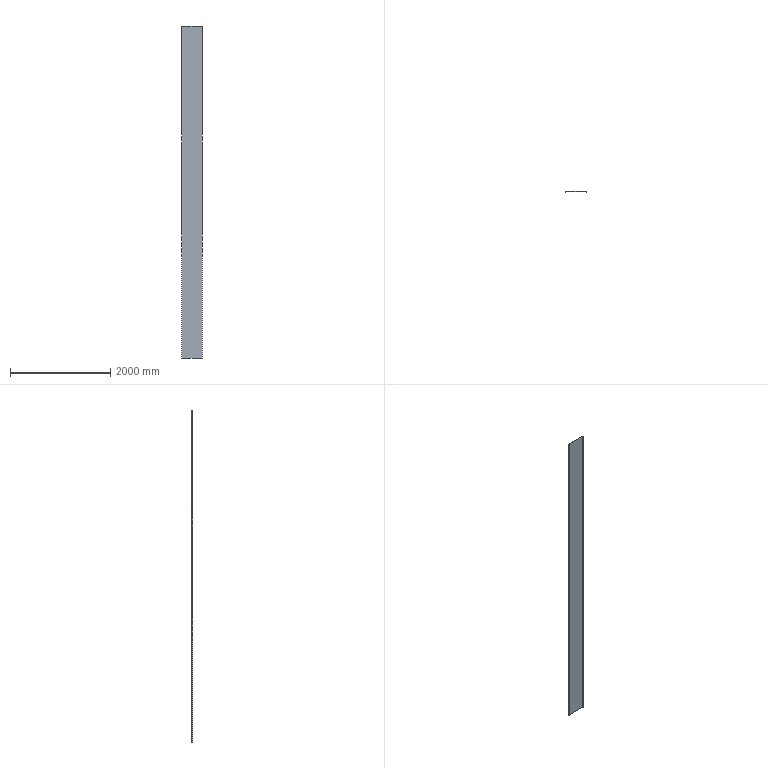Part | STEP file | 750038235 | 1 solid | 14 faces | box 405 x 21.5 x 6614 mm | volume 4395351 mm3 | plane 10 | cylinder 4 | commonest cylinder face diameters 3 x2 6 x2
STEP:
#1=CARTESIAN_POINT('',(-199.5,0.,0.));
#2=VERTEX_POINT('',#1);
#3=CARTESIAN_POINT('',(-199.5,0.,6613.5));
#4=VERTEX_POINT('',#3);
#5=CARTESIAN_POINT('',(-199.5,0.,0.));
#6=DIRECTION('',(0.,0.,1.));
#7=VECTOR('',#6,1000.);
#8=LINE('',#5,#7);
#9=EDGE_CURVE('',#2,#4,#8,.T.);
#10=ORIENTED_EDGE('',*,*,#9,.F.);
#11=CARTESIAN_POINT('',(199.5,0.,0.));
#12=VERTEX_POINT('',#11);
#13=CARTESIAN_POINT('',(201.,0.,0.));
#14=DIRECTION('',(-1.,0.,0.));
#15=VECTOR('',#14,1000.);
#16=LINE('',#13,#15);
#17=EDGE_CURVE('',#12,#2,#16,.T.);
#18=ORIENTED_EDGE('',*,*,#17,.F.);
#19=CARTESIAN_POINT('',(199.5,0.,6613.5));
#20=VERTEX_POINT('',#19);
#21=CARTESIAN_POINT('',(199.5,0.,0.));
#22=DIRECTION('',(0.,0.,-1.));
#23=VECTOR('',#22,1000.);
#24=LINE('',#21,#23);
#25=EDGE_CURVE('',#20,#12,#24,.T.);
#26=ORIENTED_EDGE('',*,*,#25,.F.);
#27=CARTESIAN_POINT('',(201.,0.,6613.5));
#28=DIRECTION('',(1.,0.,0.));
#29=VECTOR('',#28,1000.);
#30=LINE('',#27,#29);
#31=EDGE_CURVE('',#4,#20,#30,.T.);
#32=ORIENTED_EDGE('',*,*,#31,.F.);
#33=EDGE_LOOP('',(#10,#18,#26,#32));
#34=FACE_OUTER_BOUND('',#33,.T.);
#35=CARTESIAN_POINT('',(201.,0.,0.));
#36=DIRECTION('',(0.,1.,0.));
#37=DIRECTION('',(-1.,0.,0.));
#38=AXIS2_PLACEMENT_3D('',#35,#36,#37);
#39=PLANE('',#38);
#40=ADVANCED_FACE('',(#34),#39,.F.);
#41=CARTESIAN_POINT('',(201.,-20.,6613.5));
#42=VERTEX_POINT('',#41);
#43=CARTESIAN_POINT('',(202.5,-20.,6613.5));
#44=VERTEX_POINT('',#43);
#45=CARTESIAN_POINT('',(201.,-20.,6613.5));
#46=DIRECTION('',(1.,0.,0.));
#47=VECTOR('',#46,1000.);
#48=LINE('',#45,#47);
#49=EDGE_CURVE('',#42,#44,#48,.T.);
#50=ORIENTED_EDGE('',*,*,#49,.T.);
#51=CARTESIAN_POINT('',(202.5,-1.5,6613.5));
#52=VERTEX_POINT('',#51);
#53=CARTESIAN_POINT('',(202.5,-1.5,6613.5));
#54=DIRECTION('',(0.,1.,0.));
#55=VECTOR('',#54,1000.);
#56=LINE('',#53,#55);
#57=EDGE_CURVE('',#44,#52,#56,.T.);
#58=ORIENTED_EDGE('',*,*,#57,.T.);
#59=CARTESIAN_POINT('',(199.5,1.5,6613.5));
#60=VERTEX_POINT('',#59);
#61=CARTESIAN_POINT('',(199.5,-1.5,6613.5));
#62=DIRECTION('',(0.,0.,1.));
#63=DIRECTION('',(1.,0.,0.));
#64=AXIS2_PLACEMENT_3D('',#61,#62,#63);
#65=CIRCLE('',#64,3.);
#66=EDGE_CURVE('',#52,#60,#65,.T.);
#67=ORIENTED_EDGE('',*,*,#66,.T.);
#68=CARTESIAN_POINT('',(-199.5,1.5,6613.5));
#69=VERTEX_POINT('',#68);
#70=CARTESIAN_POINT('',(199.5,1.5,6613.5));
#71=DIRECTION('',(-1.,0.,0.));
#72=VECTOR('',#71,1000.);
#73=LINE('',#70,#72);
#74=EDGE_CURVE('',#60,#69,#73,.T.);
#75=ORIENTED_EDGE('',*,*,#74,.T.);
#76=CARTESIAN_POINT('',(-202.5,-1.5,6613.5));
#77=VERTEX_POINT('',#76);
#78=CARTESIAN_POINT('',(-199.5,-1.5,6613.5));
#79=DIRECTION('',(0.,0.,1.));
#80=DIRECTION('',(1.,0.,0.));
#81=AXIS2_PLACEMENT_3D('',#78,#79,#80);
#82=CIRCLE('',#81,3.);
#83=EDGE_CURVE('',#69,#77,#82,.T.);
#84=ORIENTED_EDGE('',*,*,#83,.T.);
#85=CARTESIAN_POINT('',(-202.5,-20.,6613.5));
#86=VERTEX_POINT('',#85);
#87=CARTESIAN_POINT('',(-202.5,-1.5,6613.5));
#88=DIRECTION('',(0.,-1.,0.));
#89=VECTOR('',#88,1000.);
#90=LINE('',#87,#89);
#91=EDGE_CURVE('',#77,#86,#90,.T.);
#92=ORIENTED_EDGE('',*,*,#91,.T.);
#93=CARTESIAN_POINT('',(-201.,-20.,6613.5));
#94=VERTEX_POINT('',#93);
#95=CARTESIAN_POINT('',(-201.,-20.,6613.5));
#96=DIRECTION('',(-1.,0.,0.));
#97=VECTOR('',#96,1000.);
#98=LINE('',#95,#97);
#99=EDGE_CURVE('',#94,#86,#98,.T.);
#100=ORIENTED_EDGE('',*,*,#99,.F.);
#101=CARTESIAN_POINT('',(-201.,-1.5,6613.5));
#102=VERTEX_POINT('',#101);
#103=CARTESIAN_POINT('',(-201.,-1.5,6613.5));
#104=DIRECTION('',(0.,1.,0.));
#105=VECTOR('',#104,1000.);
#106=LINE('',#103,#105);
#107=EDGE_CURVE('',#94,#102,#106,.T.);
#108=ORIENTED_EDGE('',*,*,#107,.T.);
#109=CARTESIAN_POINT('',(-199.5,-1.5,6613.5));
#110=DIRECTION('',(0.,0.,-1.));
#111=DIRECTION('',(1.,0.,0.));
#112=AXIS2_PLACEMENT_3D('',#109,#110,#111);
#113=CIRCLE('',#112,1.5);
#114=EDGE_CURVE('',#102,#4,#113,.T.);
#115=ORIENTED_EDGE('',*,*,#114,.T.);
#116=ORIENTED_EDGE('',*,*,#31,.T.);
#117=CARTESIAN_POINT('',(201.,-1.5,6613.5));
#118=VERTEX_POINT('',#117);
#119=CARTESIAN_POINT('',(199.5,-1.5,6613.5));
#120=DIRECTION('',(0.,0.,-1.));
#121=DIRECTION('',(1.,0.,0.));
#122=AXIS2_PLACEMENT_3D('',#119,#120,#121);
#123=CIRCLE('',#122,1.5);
#124=EDGE_CURVE('',#20,#118,#123,.T.);
#125=ORIENTED_EDGE('',*,*,#124,.T.);
#126=CARTESIAN_POINT('',(201.,-1.5,6613.5));
#127=DIRECTION('',(0.,-1.,0.));
#128=VECTOR('',#127,1000.);
#129=LINE('',#126,#128);
#130=EDGE_CURVE('',#118,#42,#129,.T.);
#131=ORIENTED_EDGE('',*,*,#130,.T.);
#132=EDGE_LOOP('',(#50,#58,#67,#75,#84,#92,#100,#108,#115,#116,#125,#131));
#133=FACE_OUTER_BOUND('',#132,.T.);
#134=CARTESIAN_POINT('',(199.5,-1.5,6613.5));
#135=DIRECTION('',(0.,0.,1.));
#136=DIRECTION('',(1.,0.,0.));
#137=AXIS2_PLACEMENT_3D('',#134,#135,#136);
#138=PLANE('',#137);
#139=ADVANCED_FACE('',(#133),#138,.T.);
#140=CARTESIAN_POINT('',(-201.,-1.5,0.));
#141=VERTEX_POINT('',#140);
#142=CARTESIAN_POINT('',(-201.,-1.5,0.));
#143=DIRECTION('',(0.,0.,1.));
#144=VECTOR('',#143,1000.);
#145=LINE('',#142,#144);
#146=EDGE_CURVE('',#141,#102,#145,.T.);
#147=ORIENTED_EDGE('',*,*,#146,.F.);
#148=CARTESIAN_POINT('',(-199.5,-1.5,0.));
#149=DIRECTION('',(0.,0.,1.));
#150=DIRECTION('',(1.,0.,0.));
#151=AXIS2_PLACEMENT_3D('',#148,#149,#150);
#152=CIRCLE('',#151,1.5);
#153=EDGE_CURVE('',#2,#141,#152,.T.);
#154=ORIENTED_EDGE('',*,*,#153,.F.);
#155=ORIENTED_EDGE('',*,*,#9,.T.);
#156=ORIENTED_EDGE('',*,*,#114,.F.);
#157=EDGE_LOOP('',(#147,#154,#155,#156));
#158=FACE_OUTER_BOUND('',#157,.T.);
#159=CARTESIAN_POINT('',(-199.5,-1.5,0.));
#160=DIRECTION('',(0.,0.,1.));
#161=DIRECTION('',(1.,0.,0.));
#162=AXIS2_PLACEMENT_3D('',#159,#160,#161);
#163=CYLINDRICAL_SURFACE('',#162,1.5);
#164=ADVANCED_FACE('',(#158),#163,.F.);
#165=CARTESIAN_POINT('',(202.5,-1.5,0.));
#166=VERTEX_POINT('',#165);
#167=CARTESIAN_POINT('',(202.5,-20.,0.));
#168=VERTEX_POINT('',#167);
#169=CARTESIAN_POINT('',(202.5,-20.,0.));
#170=DIRECTION('',(0.,-1.,0.));
#171=VECTOR('',#170,1000.);
#172=LINE('',#169,#171);
#173=EDGE_CURVE('',#166,#168,#172,.T.);
#174=ORIENTED_EDGE('',*,*,#173,.T.);
#175=CARTESIAN_POINT('',(201.,-20.,0.));
#176=VERTEX_POINT('',#175);
#177=CARTESIAN_POINT('',(201.,-20.,0.));
#178=DIRECTION('',(-1.,0.,0.));
#179=VECTOR('',#178,1000.);
#180=LINE('',#177,#179);
#181=EDGE_CURVE('',#168,#176,#180,.T.);
#182=ORIENTED_EDGE('',*,*,#181,.T.);
#183=CARTESIAN_POINT('',(201.,-1.5,0.));
#184=VERTEX_POINT('',#183);
#185=CARTESIAN_POINT('',(201.,-20.,0.));
#186=DIRECTION('',(0.,1.,0.));
#187=VECTOR('',#186,1000.);
#188=LINE('',#185,#187);
#189=EDGE_CURVE('',#176,#184,#188,.T.);
#190=ORIENTED_EDGE('',*,*,#189,.T.);
#191=CARTESIAN_POINT('',(199.5,-1.5,0.));
#192=DIRECTION('',(0.,0.,1.));
#193=DIRECTION('',(1.,0.,0.));
#194=AXIS2_PLACEMENT_3D('',#191,#192,#193);
#195=CIRCLE('',#194,1.5);
#196=EDGE_CURVE('',#184,#12,#195,.T.);
#197=ORIENTED_EDGE('',*,*,#196,.T.);
#198=ORIENTED_EDGE('',*,*,#17,.T.);
#199=ORIENTED_EDGE('',*,*,#153,.T.);
#200=CARTESIAN_POINT('',(-201.,-20.,0.));
#201=VERTEX_POINT('',#200);
#202=CARTESIAN_POINT('',(-201.,-20.,0.));
#203=DIRECTION('',(0.,-1.,0.));
#204=VECTOR('',#203,1000.);
#205=LINE('',#202,#204);
#206=EDGE_CURVE('',#141,#201,#205,.T.);
#207=ORIENTED_EDGE('',*,*,#206,.T.);
#208=CARTESIAN_POINT('',(-202.5,-20.,0.));
#209=VERTEX_POINT('',#208);
#210=CARTESIAN_POINT('',(-201.,-20.,0.));
#211=DIRECTION('',(1.,0.,0.));
#212=VECTOR('',#211,1000.);
#213=LINE('',#210,#212);
#214=EDGE_CURVE('',#209,#201,#213,.T.);
#215=ORIENTED_EDGE('',*,*,#214,.F.);
#216=CARTESIAN_POINT('',(-202.5,-1.5,0.));
#217=VERTEX_POINT('',#216);
#218=CARTESIAN_POINT('',(-202.5,-20.,0.));
#219=DIRECTION('',(0.,1.,0.));
#220=VECTOR('',#219,1000.);
#221=LINE('',#218,#220);
#222=EDGE_CURVE('',#209,#217,#221,.T.);
#223=ORIENTED_EDGE('',*,*,#222,.T.);
#224=CARTESIAN_POINT('',(-199.5,1.5,0.));
#225=VERTEX_POINT('',#224);
#226=CARTESIAN_POINT('',(-199.5,-1.5,0.));
#227=DIRECTION('',(0.,0.,-1.));
#228=DIRECTION('',(1.,0.,0.));
#229=AXIS2_PLACEMENT_3D('',#226,#227,#228);
#230=CIRCLE('',#229,3.);
#231=EDGE_CURVE('',#217,#225,#230,.T.);
#232=ORIENTED_EDGE('',*,*,#231,.T.);
#233=CARTESIAN_POINT('',(199.5,1.5,0.));
#234=VERTEX_POINT('',#233);
#235=CARTESIAN_POINT('',(201.,1.5,0.));
#236=DIRECTION('',(1.,0.,0.));
#237=VECTOR('',#236,1000.);
#238=LINE('',#235,#237);
#239=EDGE_CURVE('',#225,#234,#238,.T.);
#240=ORIENTED_EDGE('',*,*,#239,.T.);
#241=CARTESIAN_POINT('',(199.5,-1.5,0.));
#242=DIRECTION('',(0.,0.,-1.));
#243=DIRECTION('',(1.,0.,0.));
#244=AXIS2_PLACEMENT_3D('',#241,#242,#243);
#245=CIRCLE('',#244,3.);
#246=EDGE_CURVE('',#234,#166,#245,.T.);
#247=ORIENTED_EDGE('',*,*,#246,.T.);
#248=EDGE_LOOP('',(#174,#182,#190,#197,#198,#199,#207,#215,#223,#232,#240,#247));
#249=FACE_OUTER_BOUND('',#248,.T.);
#250=CARTESIAN_POINT('',(201.,-20.,0.));
#251=DIRECTION('',(0.,0.,-1.));
#252=DIRECTION('',(-1.,0.,0.));
#253=AXIS2_PLACEMENT_3D('',#250,#251,#252);
#254=PLANE('',#253);
#255=ADVANCED_FACE('',(#249),#254,.T.);
#256=ORIENTED_EDGE('',*,*,#25,.T.);
#257=ORIENTED_EDGE('',*,*,#196,.F.);
#258=CARTESIAN_POINT('',(201.,-1.5,0.));
#259=DIRECTION('',(0.,0.,-1.));
#260=VECTOR('',#259,1000.);
#261=LINE('',#258,#260);
#262=EDGE_CURVE('',#118,#184,#261,.T.);
#263=ORIENTED_EDGE('',*,*,#262,.F.);
#264=ORIENTED_EDGE('',*,*,#124,.F.);
#265=EDGE_LOOP('',(#256,#257,#263,#264));
#266=FACE_OUTER_BOUND('',#265,.T.);
#267=CARTESIAN_POINT('',(199.5,-1.5,0.));
#268=DIRECTION('',(0.,0.,1.));
#269=DIRECTION('',(1.,0.,0.));
#270=AXIS2_PLACEMENT_3D('',#267,#268,#269);
#271=CYLINDRICAL_SURFACE('',#270,1.5);
#272=ADVANCED_FACE('',(#266),#271,.F.);
#273=ORIENTED_EDGE('',*,*,#173,.F.);
#274=CARTESIAN_POINT('',(202.5,-1.5,0.));
#275=DIRECTION('',(0.,0.,1.));
#276=VECTOR('',#275,1000.);
#277=LINE('',#274,#276);
#278=EDGE_CURVE('',#166,#52,#277,.T.);
#279=ORIENTED_EDGE('',*,*,#278,.T.);
#280=ORIENTED_EDGE('',*,*,#57,.F.);
#281=CARTESIAN_POINT('',(202.5,-20.,0.));
#282=DIRECTION('',(0.,0.,-1.));
#283=VECTOR('',#282,1000.);
#284=LINE('',#281,#283);
#285=EDGE_CURVE('',#44,#168,#284,.T.);
#286=ORIENTED_EDGE('',*,*,#285,.T.);
#287=EDGE_LOOP('',(#273,#279,#280,#286));
#288=FACE_OUTER_BOUND('',#287,.T.);
#289=CARTESIAN_POINT('',(202.5,-20.,0.));
#290=DIRECTION('',(1.,0.,0.));
#291=DIRECTION('',(0.,0.,-1.));
#292=AXIS2_PLACEMENT_3D('',#289,#290,#291);
#293=PLANE('',#292);
#294=ADVANCED_FACE('',(#288),#293,.T.);
#295=ORIENTED_EDGE('',*,*,#262,.T.);
#296=ORIENTED_EDGE('',*,*,#189,.F.);
#297=CARTESIAN_POINT('',(201.,-20.,0.));
#298=DIRECTION('',(0.,0.,-1.));
#299=VECTOR('',#298,1000.);
#300=LINE('',#297,#299);
#301=EDGE_CURVE('',#42,#176,#300,.T.);
#302=ORIENTED_EDGE('',*,*,#301,.F.);
#303=ORIENTED_EDGE('',*,*,#130,.F.);
#304=EDGE_LOOP('',(#295,#296,#302,#303));
#305=FACE_OUTER_BOUND('',#304,.T.);
#306=CARTESIAN_POINT('',(201.,-20.,0.));
#307=DIRECTION('',(1.,0.,0.));
#308=DIRECTION('',(0.,0.,-1.));
#309=AXIS2_PLACEMENT_3D('',#306,#307,#308);
#310=PLANE('',#309);
#311=ADVANCED_FACE('',(#305),#310,.F.);
#312=CARTESIAN_POINT('',(-201.,-20.,0.));
#313=DIRECTION('',(0.,0.,1.));
#314=VECTOR('',#313,1000.);
#315=LINE('',#312,#314);
#316=EDGE_CURVE('',#201,#94,#315,.T.);
#317=ORIENTED_EDGE('',*,*,#316,.F.);
#318=ORIENTED_EDGE('',*,*,#206,.F.);
#319=ORIENTED_EDGE('',*,*,#146,.T.);
#320=ORIENTED_EDGE('',*,*,#107,.F.);
#321=EDGE_LOOP('',(#317,#318,#319,#320));
#322=FACE_OUTER_BOUND('',#321,.T.);
#323=CARTESIAN_POINT('',(-201.,0.,0.));
#324=DIRECTION('',(-1.,0.,0.));
#325=DIRECTION('',(0.,0.,1.));
#326=AXIS2_PLACEMENT_3D('',#323,#324,#325);
#327=PLANE('',#326);
#328=ADVANCED_FACE('',(#322),#327,.F.);
#329=ORIENTED_EDGE('',*,*,#222,.F.);
#330=CARTESIAN_POINT('',(-202.5,-20.,0.));
#331=DIRECTION('',(0.,0.,1.));
#332=VECTOR('',#331,1000.);
#333=LINE('',#330,#332);
#334=EDGE_CURVE('',#209,#86,#333,.T.);
#335=ORIENTED_EDGE('',*,*,#334,.T.);
#336=ORIENTED_EDGE('',*,*,#91,.F.);
#337=CARTESIAN_POINT('',(-202.5,-1.5,0.));
#338=DIRECTION('',(0.,0.,-1.));
#339=VECTOR('',#338,1000.);
#340=LINE('',#337,#339);
#341=EDGE_CURVE('',#77,#217,#340,.T.);
#342=ORIENTED_EDGE('',*,*,#341,.T.);
#343=EDGE_LOOP('',(#329,#335,#336,#342));
#344=FACE_OUTER_BOUND('',#343,.T.);
#345=CARTESIAN_POINT('',(-202.5,0.,0.));
#346=DIRECTION('',(-1.,0.,0.));
#347=DIRECTION('',(0.,0.,1.));
#348=AXIS2_PLACEMENT_3D('',#345,#346,#347);
#349=PLANE('',#348);
#350=ADVANCED_FACE('',(#344),#349,.T.);
#351=ORIENTED_EDGE('',*,*,#231,.F.);
#352=ORIENTED_EDGE('',*,*,#341,.F.);
#353=ORIENTED_EDGE('',*,*,#83,.F.);
#354=CARTESIAN_POINT('',(-199.5,1.5,0.));
#355=DIRECTION('',(0.,0.,-1.));
#356=VECTOR('',#355,1000.);
#357=LINE('',#354,#356);
#358=EDGE_CURVE('',#69,#225,#357,.T.);
#359=ORIENTED_EDGE('',*,*,#358,.T.);
#360=EDGE_LOOP('',(#351,#352,#353,#359));
#361=FACE_OUTER_BOUND('',#360,.T.);
#362=CARTESIAN_POINT('',(-199.5,-1.5,0.));
#363=DIRECTION('',(0.,0.,1.));
#364=DIRECTION('',(1.,0.,0.));
#365=AXIS2_PLACEMENT_3D('',#362,#363,#364);
#366=CYLINDRICAL_SURFACE('',#365,3.);
#367=ADVANCED_FACE('',(#361),#366,.T.);
#368=ORIENTED_EDGE('',*,*,#239,.F.);
#369=ORIENTED_EDGE('',*,*,#358,.F.);
#370=ORIENTED_EDGE('',*,*,#74,.F.);
#371=CARTESIAN_POINT('',(199.5,1.5,0.));
#372=DIRECTION('',(0.,0.,-1.));
#373=VECTOR('',#372,1000.);
#374=LINE('',#371,#373);
#375=EDGE_CURVE('',#60,#234,#374,.T.);
#376=ORIENTED_EDGE('',*,*,#375,.T.);
#377=EDGE_LOOP('',(#368,#369,#370,#376));
#378=FACE_OUTER_BOUND('',#377,.T.);
#379=CARTESIAN_POINT('',(201.,1.5,0.));
#380=DIRECTION('',(0.,1.,0.));
#381=DIRECTION('',(-1.,0.,0.));
#382=AXIS2_PLACEMENT_3D('',#379,#380,#381);
#383=PLANE('',#382);
#384=ADVANCED_FACE('',(#378),#383,.T.);
#385=ORIENTED_EDGE('',*,*,#246,.F.);
#386=ORIENTED_EDGE('',*,*,#375,.F.);
#387=ORIENTED_EDGE('',*,*,#66,.F.);
#388=ORIENTED_EDGE('',*,*,#278,.F.);
#389=EDGE_LOOP('',(#385,#386,#387,#388));
#390=FACE_OUTER_BOUND('',#389,.T.);
#391=CARTESIAN_POINT('',(199.5,-1.5,0.));
#392=DIRECTION('',(0.,0.,1.));
#393=DIRECTION('',(1.,0.,0.));
#394=AXIS2_PLACEMENT_3D('',#391,#392,#393);
#395=CYLINDRICAL_SURFACE('',#394,3.);
#396=ADVANCED_FACE('',(#390),#395,.T.);
#397=ORIENTED_EDGE('',*,*,#285,.F.);
#398=ORIENTED_EDGE('',*,*,#49,.F.);
#399=ORIENTED_EDGE('',*,*,#301,.T.);
#400=ORIENTED_EDGE('',*,*,#181,.F.);
#401=EDGE_LOOP('',(#397,#398,#399,#400));
#402=FACE_OUTER_BOUND('',#401,.T.);
#403=CARTESIAN_POINT('',(201.,-20.,0.));
#404=DIRECTION('',(0.,1.,0.));
#405=DIRECTION('',(0.,0.,1.));
#406=AXIS2_PLACEMENT_3D('',#403,#404,#405);
#407=PLANE('',#406);
#408=ADVANCED_FACE('',(#402),#407,.F.);
#409=ORIENTED_EDGE('',*,*,#214,.T.);
#410=ORIENTED_EDGE('',*,*,#316,.T.);
#411=ORIENTED_EDGE('',*,*,#99,.T.);
#412=ORIENTED_EDGE('',*,*,#334,.F.);
#413=EDGE_LOOP('',(#409,#410,#411,#412));
#414=FACE_OUTER_BOUND('',#413,.T.);
#415=CARTESIAN_POINT('',(-201.,-20.,0.));
#416=DIRECTION('',(0.,-1.,0.));
#417=DIRECTION('',(0.,0.,-1.));
#418=AXIS2_PLACEMENT_3D('',#415,#416,#417);
#419=PLANE('',#418);
#420=ADVANCED_FACE('',(#414),#419,.T.);
#421=CLOSED_SHELL('',(#40,#139,#164,#255,#272,#294,#311,#328,#350,#367,#384,#396,#408,#420));
#422=MANIFOLD_SOLID_BREP('',#421);
#423=CARTESIAN_POINT('',(0.,0.,0.));
#424=DIRECTION('',(0.,0.,1.));
#425=DIRECTION('',(1.,0.,0.));
#426=AXIS2_PLACEMENT_3D('',#423,#424,#425);
#427=(LENGTH_UNIT()NAMED_UNIT(*)SI_UNIT(.MILLI.,.METRE.));
#428=UNCERTAINTY_MEASURE_WITH_UNIT(LENGTH_MEASURE(0.00001),#427,'','');
#429=(NAMED_UNIT(*)PLANE_ANGLE_UNIT()SI_UNIT($,.RADIAN.));
#430=(NAMED_UNIT(*)SI_UNIT($,.STERADIAN.)SOLID_ANGLE_UNIT());
#431=(GEOMETRIC_REPRESENTATION_CONTEXT(3)GLOBAL_UNCERTAINTY_ASSIGNED_CONTEXT((#428))GLOBAL_UNIT_ASSIGNED_CONTEXT((#427,#429,#430))REPRESENTATION_CONTEXT('',''));
#432=ADVANCED_BREP_SHAPE_REPRESENTATION('',(#422,#426),#431);